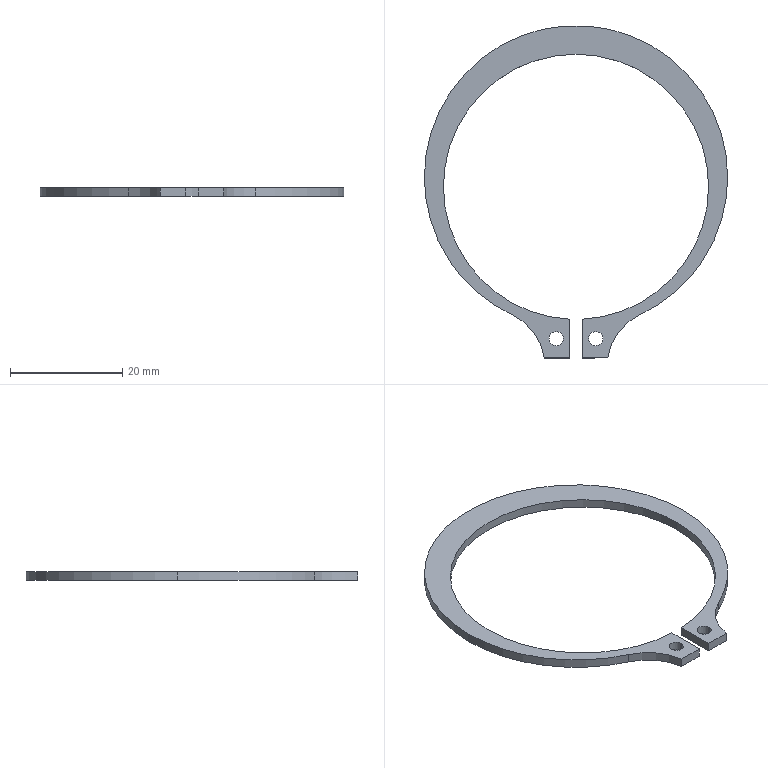Part | SolidWorks | features BaseBody 1 | 1 solid | 18 faces | box 54 x 59.172 x 1.6 mm | volume 946.092 mm3 | cylinder 12 | plane 6 | commonest cylinder face diameters 2.5 x4 47.2 x3 54 x3 19.938 x2
STEP:
#1=CARTESIAN_POINT('',(4.775,-27.022,0.));
#2=VERTEX_POINT('',#1);
#3=CARTESIAN_POINT('',(2.275,-27.022,0.));
#4=VERTEX_POINT('',#3);
#5=CARTESIAN_POINT('',(3.525,-27.022,0.));
#6=DIRECTION('',(0.,0.,-1.));
#7=DIRECTION('',(-1.,0.,0.));
#8=AXIS2_PLACEMENT_3D('',#5,#6,#7);
#9=CIRCLE('',#8,1.25);
#10=EDGE_CURVE('',#2,#4,#9,.T.);
#11=ORIENTED_EDGE('',*,*,#10,.F.);
#12=CARTESIAN_POINT('',(4.775,-27.022,-1.6));
#13=VERTEX_POINT('',#12);
#14=CARTESIAN_POINT('',(4.775,-27.022,0.));
#15=DIRECTION('',(0.,0.,-1.));
#16=VECTOR('',#15,1000.);
#17=LINE('',#14,#16);
#18=EDGE_CURVE('',#2,#13,#17,.T.);
#19=ORIENTED_EDGE('',*,*,#18,.T.);
#20=CARTESIAN_POINT('',(2.275,-27.022,-1.6));
#21=VERTEX_POINT('',#20);
#22=CARTESIAN_POINT('',(3.525,-27.022,-1.6));
#23=DIRECTION('',(0.,0.,-1.));
#24=DIRECTION('',(-1.,0.,0.));
#25=AXIS2_PLACEMENT_3D('',#22,#23,#24);
#26=CIRCLE('',#25,1.25);
#27=EDGE_CURVE('',#13,#21,#26,.T.);
#28=ORIENTED_EDGE('',*,*,#27,.T.);
#29=CARTESIAN_POINT('',(2.275,-27.022,0.));
#30=DIRECTION('',(0.,0.,-1.));
#31=VECTOR('',#30,1000.);
#32=LINE('',#29,#31);
#33=EDGE_CURVE('',#4,#21,#32,.T.);
#34=ORIENTED_EDGE('',*,*,#33,.F.);
#35=EDGE_LOOP('',(#11,#19,#28,#34));
#36=FACE_OUTER_BOUND('',#35,.T.);
#37=CARTESIAN_POINT('',(3.525,-27.022,0.));
#38=DIRECTION('',(0.,0.,-1.));
#39=DIRECTION('',(-1.,0.,0.));
#40=AXIS2_PLACEMENT_3D('',#37,#38,#39);
#41=CYLINDRICAL_SURFACE('',#40,1.25);
#42=ADVANCED_FACE('',(#36),#41,.F.);
#43=CARTESIAN_POINT('',(-2.275,-27.022,0.));
#44=VERTEX_POINT('',#43);
#45=CARTESIAN_POINT('',(-4.775,-27.022,0.));
#46=VERTEX_POINT('',#45);
#47=CARTESIAN_POINT('',(-3.525,-27.022,0.));
#48=DIRECTION('',(0.,0.,-1.));
#49=DIRECTION('',(-1.,0.,0.));
#50=AXIS2_PLACEMENT_3D('',#47,#48,#49);
#51=CIRCLE('',#50,1.25);
#52=EDGE_CURVE('',#44,#46,#51,.T.);
#53=ORIENTED_EDGE('',*,*,#52,.F.);
#54=CARTESIAN_POINT('',(-2.275,-27.022,-1.6));
#55=VERTEX_POINT('',#54);
#56=CARTESIAN_POINT('',(-2.275,-27.022,0.));
#57=DIRECTION('',(0.,0.,-1.));
#58=VECTOR('',#57,1000.);
#59=LINE('',#56,#58);
#60=EDGE_CURVE('',#44,#55,#59,.T.);
#61=ORIENTED_EDGE('',*,*,#60,.T.);
#62=CARTESIAN_POINT('',(-4.775,-27.022,-1.6));
#63=VERTEX_POINT('',#62);
#64=CARTESIAN_POINT('',(-3.525,-27.022,-1.6));
#65=DIRECTION('',(0.,0.,-1.));
#66=DIRECTION('',(-1.,0.,0.));
#67=AXIS2_PLACEMENT_3D('',#64,#65,#66);
#68=CIRCLE('',#67,1.25);
#69=EDGE_CURVE('',#55,#63,#68,.T.);
#70=ORIENTED_EDGE('',*,*,#69,.T.);
#71=CARTESIAN_POINT('',(-4.775,-27.022,0.));
#72=DIRECTION('',(0.,0.,-1.));
#73=VECTOR('',#72,1000.);
#74=LINE('',#71,#73);
#75=EDGE_CURVE('',#46,#63,#74,.T.);
#76=ORIENTED_EDGE('',*,*,#75,.F.);
#77=EDGE_LOOP('',(#53,#61,#70,#76));
#78=FACE_OUTER_BOUND('',#77,.T.);
#79=CARTESIAN_POINT('',(-3.525,-27.022,0.));
#80=DIRECTION('',(0.,0.,-1.));
#81=DIRECTION('',(-1.,0.,0.));
#82=AXIS2_PLACEMENT_3D('',#79,#80,#81);
#83=CYLINDRICAL_SURFACE('',#82,1.25);
#84=ADVANCED_FACE('',(#78),#83,.F.);
#85=CARTESIAN_POINT('',(-27.,1.7,0.));
#86=VERTEX_POINT('',#85);
#87=CARTESIAN_POINT('',(27.,1.7,0.));
#88=VERTEX_POINT('',#87);
#89=CARTESIAN_POINT('',(0.,1.7,0.));
#90=DIRECTION('',(0.,0.,-1.));
#91=DIRECTION('',(-1.,0.,0.));
#92=AXIS2_PLACEMENT_3D('',#89,#90,#91);
#93=CIRCLE('',#92,27.);
#94=EDGE_CURVE('',#86,#88,#93,.T.);
#95=ORIENTED_EDGE('',*,*,#94,.T.);
#96=CARTESIAN_POINT('',(27.,1.7,-1.6));
#97=VERTEX_POINT('',#96);
#98=CARTESIAN_POINT('',(27.,1.7,0.));
#99=DIRECTION('',(0.,0.,-1.));
#100=VECTOR('',#99,1000.);
#101=LINE('',#98,#100);
#102=EDGE_CURVE('',#88,#97,#101,.T.);
#103=ORIENTED_EDGE('',*,*,#102,.T.);
#104=CARTESIAN_POINT('',(-27.,1.7,-1.6));
#105=VERTEX_POINT('',#104);
#106=CARTESIAN_POINT('',(0.,1.7,-1.6));
#107=DIRECTION('',(0.,0.,1.));
#108=DIRECTION('',(-1.,0.,0.));
#109=AXIS2_PLACEMENT_3D('',#106,#107,#108);
#110=CIRCLE('',#109,27.);
#111=EDGE_CURVE('',#97,#105,#110,.T.);
#112=ORIENTED_EDGE('',*,*,#111,.T.);
#113=CARTESIAN_POINT('',(-27.,1.7,0.));
#114=DIRECTION('',(0.,0.,-1.));
#115=VECTOR('',#114,1000.);
#116=LINE('',#113,#115);
#117=EDGE_CURVE('',#86,#105,#116,.T.);
#118=ORIENTED_EDGE('',*,*,#117,.F.);
#119=EDGE_LOOP('',(#95,#103,#112,#118));
#120=FACE_OUTER_BOUND('',#119,.T.);
#121=CARTESIAN_POINT('',(0.,1.7,0.));
#122=DIRECTION('',(0.,0.,-1.));
#123=DIRECTION('',(-1.,0.,0.));
#124=AXIS2_PLACEMENT_3D('',#121,#122,#123);
#125=CYLINDRICAL_SURFACE('',#124,27.);
#126=ADVANCED_FACE('',(#120),#125,.T.);
#127=CARTESIAN_POINT('',(-11.337,-22.805,0.));
#128=VERTEX_POINT('',#127);
#129=CARTESIAN_POINT('',(0.,1.7,0.));
#130=DIRECTION('',(0.,0.,-1.));
#131=DIRECTION('',(-1.,0.,0.));
#132=AXIS2_PLACEMENT_3D('',#129,#130,#131);
#133=CIRCLE('',#132,27.);
#134=EDGE_CURVE('',#128,#86,#133,.T.);
#135=ORIENTED_EDGE('',*,*,#134,.T.);
#136=ORIENTED_EDGE('',*,*,#117,.T.);
#137=CARTESIAN_POINT('',(-11.337,-22.805,-1.6));
#138=VERTEX_POINT('',#137);
#139=CARTESIAN_POINT('',(0.,1.7,-1.6));
#140=DIRECTION('',(0.,0.,1.));
#141=DIRECTION('',(-1.,0.,0.));
#142=AXIS2_PLACEMENT_3D('',#139,#140,#141);
#143=CIRCLE('',#142,27.);
#144=EDGE_CURVE('',#105,#138,#143,.T.);
#145=ORIENTED_EDGE('',*,*,#144,.T.);
#146=CARTESIAN_POINT('',(-11.337,-22.805,0.));
#147=DIRECTION('',(0.,0.,1.));
#148=VECTOR('',#147,1000.);
#149=LINE('',#146,#148);
#150=EDGE_CURVE('',#138,#128,#149,.T.);
#151=ORIENTED_EDGE('',*,*,#150,.T.);
#152=EDGE_LOOP('',(#135,#136,#145,#151));
#153=FACE_OUTER_BOUND('',#152,.T.);
#154=CARTESIAN_POINT('',(0.,1.7,0.));
#155=DIRECTION('',(0.,0.,-1.));
#156=DIRECTION('',(-1.,0.,0.));
#157=AXIS2_PLACEMENT_3D('',#154,#155,#156);
#158=CYLINDRICAL_SURFACE('',#157,27.);
#159=ADVANCED_FACE('',(#153),#158,.T.);
#160=CARTESIAN_POINT('',(23.6,0.,0.));
#161=VERTEX_POINT('',#160);
#162=CARTESIAN_POINT('',(1.15,-23.572,0.));
#163=VERTEX_POINT('',#162);
#164=CARTESIAN_POINT('',(0.,0.,0.));
#165=DIRECTION('',(0.,0.,-1.));
#166=DIRECTION('',(-1.,0.,0.));
#167=AXIS2_PLACEMENT_3D('',#164,#165,#166);
#168=CIRCLE('',#167,23.6);
#169=EDGE_CURVE('',#161,#163,#168,.T.);
#170=ORIENTED_EDGE('',*,*,#169,.F.);
#171=CARTESIAN_POINT('',(23.6,0.,-1.6));
#172=VERTEX_POINT('',#171);
#173=CARTESIAN_POINT('',(23.6,0.,0.));
#174=DIRECTION('',(0.,0.,-1.));
#175=VECTOR('',#174,1000.);
#176=LINE('',#173,#175);
#177=EDGE_CURVE('',#161,#172,#176,.T.);
#178=ORIENTED_EDGE('',*,*,#177,.T.);
#179=CARTESIAN_POINT('',(1.15,-23.572,-1.6));
#180=VERTEX_POINT('',#179);
#181=CARTESIAN_POINT('',(0.,0.,-1.6));
#182=DIRECTION('',(0.,0.,-1.));
#183=DIRECTION('',(-1.,0.,0.));
#184=AXIS2_PLACEMENT_3D('',#181,#182,#183);
#185=CIRCLE('',#184,23.6);
#186=EDGE_CURVE('',#172,#180,#185,.T.);
#187=ORIENTED_EDGE('',*,*,#186,.T.);
#188=CARTESIAN_POINT('',(1.15,-23.572,0.));
#189=DIRECTION('',(0.,0.,-1.));
#190=VECTOR('',#189,1000.);
#191=LINE('',#188,#190);
#192=EDGE_CURVE('',#163,#180,#191,.T.);
#193=ORIENTED_EDGE('',*,*,#192,.F.);
#194=EDGE_LOOP('',(#170,#178,#187,#193));
#195=FACE_OUTER_BOUND('',#194,.T.);
#196=CARTESIAN_POINT('',(0.,0.,0.));
#197=DIRECTION('',(0.,0.,-1.));
#198=DIRECTION('',(-1.,0.,0.));
#199=AXIS2_PLACEMENT_3D('',#196,#197,#198);
#200=CYLINDRICAL_SURFACE('',#199,23.6);
#201=ADVANCED_FACE('',(#195),#200,.F.);
#202=ORIENTED_EDGE('',*,*,#177,.F.);
#203=CARTESIAN_POINT('',(-23.6,0.,0.));
#204=VERTEX_POINT('',#203);
#205=CARTESIAN_POINT('',(0.,0.,0.));
#206=DIRECTION('',(0.,0.,-1.));
#207=DIRECTION('',(-1.,0.,0.));
#208=AXIS2_PLACEMENT_3D('',#205,#206,#207);
#209=CIRCLE('',#208,23.6);
#210=EDGE_CURVE('',#204,#161,#209,.T.);
#211=ORIENTED_EDGE('',*,*,#210,.F.);
#212=CARTESIAN_POINT('',(-23.6,0.,-1.6));
#213=VERTEX_POINT('',#212);
#214=CARTESIAN_POINT('',(-23.6,0.,0.));
#215=DIRECTION('',(0.,0.,-1.));
#216=VECTOR('',#215,1000.);
#217=LINE('',#214,#216);
#218=EDGE_CURVE('',#204,#213,#217,.T.);
#219=ORIENTED_EDGE('',*,*,#218,.T.);
#220=CARTESIAN_POINT('',(0.,0.,-1.6));
#221=DIRECTION('',(0.,0.,-1.));
#222=DIRECTION('',(-1.,0.,0.));
#223=AXIS2_PLACEMENT_3D('',#220,#221,#222);
#224=CIRCLE('',#223,23.6);
#225=EDGE_CURVE('',#213,#172,#224,.T.);
#226=ORIENTED_EDGE('',*,*,#225,.T.);
#227=EDGE_LOOP('',(#202,#211,#219,#226));
#228=FACE_OUTER_BOUND('',#227,.T.);
#229=CARTESIAN_POINT('',(0.,0.,0.));
#230=DIRECTION('',(0.,0.,-1.));
#231=DIRECTION('',(-1.,0.,0.));
#232=AXIS2_PLACEMENT_3D('',#229,#230,#231);
#233=CYLINDRICAL_SURFACE('',#232,23.6);
#234=ADVANCED_FACE('',(#228),#233,.F.);
#235=CARTESIAN_POINT('',(3.525,-27.022,-1.6));
#236=DIRECTION('',(0.,0.,-1.));
#237=DIRECTION('',(-1.,0.,0.));
#238=AXIS2_PLACEMENT_3D('',#235,#236,#237);
#239=CIRCLE('',#238,1.25);
#240=EDGE_CURVE('',#21,#13,#239,.T.);
#241=ORIENTED_EDGE('',*,*,#240,.F.);
#242=ORIENTED_EDGE('',*,*,#27,.F.);
#243=EDGE_LOOP('',(#241,#242));
#244=FACE_BOUND('',#243,.T.);
#245=CARTESIAN_POINT('',(-3.525,-27.022,-1.6));
#246=DIRECTION('',(0.,0.,-1.));
#247=DIRECTION('',(-1.,0.,0.));
#248=AXIS2_PLACEMENT_3D('',#245,#246,#247);
#249=CIRCLE('',#248,1.25);
#250=EDGE_CURVE('',#63,#55,#249,.T.);
#251=ORIENTED_EDGE('',*,*,#250,.F.);
#252=ORIENTED_EDGE('',*,*,#69,.F.);
#253=EDGE_LOOP('',(#251,#252));
#254=FACE_BOUND('',#253,.T.);
#255=CARTESIAN_POINT('',(-5.65,-30.472,-1.6));
#256=VERTEX_POINT('',#255);
#257=CARTESIAN_POINT('',(-1.15,-30.472,-1.6));
#258=VERTEX_POINT('',#257);
#259=CARTESIAN_POINT('',(0.,-30.472,-1.6));
#260=DIRECTION('',(1.,0.,0.));
#261=VECTOR('',#260,1000.);
#262=LINE('',#259,#261);
#263=EDGE_CURVE('',#256,#258,#262,.T.);
#264=ORIENTED_EDGE('',*,*,#263,.F.);
#265=CARTESIAN_POINT('',(-15.523,-31.852,-1.6));
#266=DIRECTION('',(0.,0.,-1.));
#267=DIRECTION('',(-1.,0.,0.));
#268=AXIS2_PLACEMENT_3D('',#265,#266,#267);
#269=CIRCLE('',#268,9.969);
#270=EDGE_CURVE('',#138,#256,#269,.T.);
#271=ORIENTED_EDGE('',*,*,#270,.F.);
#272=ORIENTED_EDGE('',*,*,#144,.F.);
#273=ORIENTED_EDGE('',*,*,#111,.F.);
#274=CARTESIAN_POINT('',(11.337,-22.805,-1.6));
#275=VERTEX_POINT('',#274);
#276=CARTESIAN_POINT('',(0.,1.7,-1.6));
#277=DIRECTION('',(0.,0.,1.));
#278=DIRECTION('',(-1.,0.,0.));
#279=AXIS2_PLACEMENT_3D('',#276,#277,#278);
#280=CIRCLE('',#279,27.);
#281=EDGE_CURVE('',#275,#97,#280,.T.);
#282=ORIENTED_EDGE('',*,*,#281,.F.);
#283=CARTESIAN_POINT('',(5.65,-30.472,-1.6));
#284=VERTEX_POINT('',#283);
#285=CARTESIAN_POINT('',(15.523,-31.852,-1.6));
#286=DIRECTION('',(0.,0.,-1.));
#287=DIRECTION('',(-1.,0.,0.));
#288=AXIS2_PLACEMENT_3D('',#285,#286,#287);
#289=CIRCLE('',#288,9.969);
#290=EDGE_CURVE('',#284,#275,#289,.T.);
#291=ORIENTED_EDGE('',*,*,#290,.F.);
#292=CARTESIAN_POINT('',(1.15,-30.472,-1.6));
#293=VERTEX_POINT('',#292);
#294=CARTESIAN_POINT('',(0.,-30.472,-1.6));
#295=DIRECTION('',(1.,0.,0.));
#296=VECTOR('',#295,1000.);
#297=LINE('',#294,#296);
#298=EDGE_CURVE('',#293,#284,#297,.T.);
#299=ORIENTED_EDGE('',*,*,#298,.F.);
#300=CARTESIAN_POINT('',(1.15,-2.891,-1.6));
#301=DIRECTION('',(0.,-1.,0.));
#302=VECTOR('',#301,1000.);
#303=LINE('',#300,#302);
#304=EDGE_CURVE('',#180,#293,#303,.T.);
#305=ORIENTED_EDGE('',*,*,#304,.F.);
#306=ORIENTED_EDGE('',*,*,#186,.F.);
#307=ORIENTED_EDGE('',*,*,#225,.F.);
#308=CARTESIAN_POINT('',(-1.15,-23.572,-1.6));
#309=VERTEX_POINT('',#308);
#310=CARTESIAN_POINT('',(0.,0.,-1.6));
#311=DIRECTION('',(0.,0.,-1.));
#312=DIRECTION('',(-1.,0.,0.));
#313=AXIS2_PLACEMENT_3D('',#310,#311,#312);
#314=CIRCLE('',#313,23.6);
#315=EDGE_CURVE('',#309,#213,#314,.T.);
#316=ORIENTED_EDGE('',*,*,#315,.F.);
#317=CARTESIAN_POINT('',(-1.15,-2.891,-1.6));
#318=DIRECTION('',(0.,1.,0.));
#319=VECTOR('',#318,1000.);
#320=LINE('',#317,#319);
#321=EDGE_CURVE('',#258,#309,#320,.T.);
#322=ORIENTED_EDGE('',*,*,#321,.F.);
#323=EDGE_LOOP('',(#264,#271,#272,#273,#282,#291,#299,#305,#306,#307,#316,#322));
#324=FACE_OUTER_BOUND('',#323,.T.);
#325=CARTESIAN_POINT('',(0.,-2.891,-1.6));
#326=DIRECTION('',(0.,0.,1.));
#327=DIRECTION('',(1.,0.,0.));
#328=AXIS2_PLACEMENT_3D('',#325,#326,#327);
#329=PLANE('',#328);
#330=ADVANCED_FACE('',(#244,#254,#324),#329,.F.);
#331=ORIENTED_EDGE('',*,*,#18,.F.);
#332=CARTESIAN_POINT('',(3.525,-27.022,0.));
#333=DIRECTION('',(0.,0.,-1.));
#334=DIRECTION('',(-1.,0.,0.));
#335=AXIS2_PLACEMENT_3D('',#332,#333,#334);
#336=CIRCLE('',#335,1.25);
#337=EDGE_CURVE('',#4,#2,#336,.T.);
#338=ORIENTED_EDGE('',*,*,#337,.F.);
#339=ORIENTED_EDGE('',*,*,#33,.T.);
#340=ORIENTED_EDGE('',*,*,#240,.T.);
#341=EDGE_LOOP('',(#331,#338,#339,#340));
#342=FACE_OUTER_BOUND('',#341,.T.);
#343=CARTESIAN_POINT('',(3.525,-27.022,0.));
#344=DIRECTION('',(0.,0.,-1.));
#345=DIRECTION('',(-1.,0.,0.));
#346=AXIS2_PLACEMENT_3D('',#343,#344,#345);
#347=CYLINDRICAL_SURFACE('',#346,1.25);
#348=ADVANCED_FACE('',(#342),#347,.F.);
#349=ORIENTED_EDGE('',*,*,#60,.F.);
#350=CARTESIAN_POINT('',(-3.525,-27.022,0.));
#351=DIRECTION('',(0.,0.,-1.));
#352=DIRECTION('',(-1.,0.,0.));
#353=AXIS2_PLACEMENT_3D('',#350,#351,#352);
#354=CIRCLE('',#353,1.25);
#355=EDGE_CURVE('',#46,#44,#354,.T.);
#356=ORIENTED_EDGE('',*,*,#355,.F.);
#357=ORIENTED_EDGE('',*,*,#75,.T.);
#358=ORIENTED_EDGE('',*,*,#250,.T.);
#359=EDGE_LOOP('',(#349,#356,#357,#358));
#360=FACE_OUTER_BOUND('',#359,.T.);
#361=CARTESIAN_POINT('',(-3.525,-27.022,0.));
#362=DIRECTION('',(0.,0.,-1.));
#363=DIRECTION('',(-1.,0.,0.));
#364=AXIS2_PLACEMENT_3D('',#361,#362,#363);
#365=CYLINDRICAL_SURFACE('',#364,1.25);
#366=ADVANCED_FACE('',(#360),#365,.F.);
#367=CARTESIAN_POINT('',(-1.15,-23.572,0.));
#368=VERTEX_POINT('',#367);
#369=CARTESIAN_POINT('',(-1.15,-30.472,0.));
#370=VERTEX_POINT('',#369);
#371=CARTESIAN_POINT('',(-1.15,-30.472,0.));
#372=DIRECTION('',(0.,-1.,0.));
#373=VECTOR('',#372,1000.);
#374=LINE('',#371,#373);
#375=EDGE_CURVE('',#368,#370,#374,.T.);
#376=ORIENTED_EDGE('',*,*,#375,.T.);
#377=CARTESIAN_POINT('',(-1.15,-30.472,0.));
#378=DIRECTION('',(0.,0.,-1.));
#379=VECTOR('',#378,1000.);
#380=LINE('',#377,#379);
#381=EDGE_CURVE('',#370,#258,#380,.T.);
#382=ORIENTED_EDGE('',*,*,#381,.T.);
#383=ORIENTED_EDGE('',*,*,#321,.T.);
#384=CARTESIAN_POINT('',(-1.15,-23.572,0.));
#385=DIRECTION('',(0.,0.,1.));
#386=VECTOR('',#385,1000.);
#387=LINE('',#384,#386);
#388=EDGE_CURVE('',#309,#368,#387,.T.);
#389=ORIENTED_EDGE('',*,*,#388,.T.);
#390=EDGE_LOOP('',(#376,#382,#383,#389));
#391=FACE_OUTER_BOUND('',#390,.T.);
#392=CARTESIAN_POINT('',(-1.15,-30.472,0.));
#393=DIRECTION('',(1.,0.,0.));
#394=DIRECTION('',(0.,1.,0.));
#395=AXIS2_PLACEMENT_3D('',#392,#393,#394);
#396=PLANE('',#395);
#397=ADVANCED_FACE('',(#391),#396,.T.);
#398=CARTESIAN_POINT('',(-5.65,-30.472,0.));
#399=VERTEX_POINT('',#398);
#400=CARTESIAN_POINT('',(-5.65,-30.472,0.));
#401=DIRECTION('',(-1.,0.,0.));
#402=VECTOR('',#401,1000.);
#403=LINE('',#400,#402);
#404=EDGE_CURVE('',#370,#399,#403,.T.);
#405=ORIENTED_EDGE('',*,*,#404,.T.);
#406=CARTESIAN_POINT('',(-5.65,-30.472,0.));
#407=DIRECTION('',(0.,0.,-1.));
#408=VECTOR('',#407,1000.);
#409=LINE('',#406,#408);
#410=EDGE_CURVE('',#399,#256,#409,.T.);
#411=ORIENTED_EDGE('',*,*,#410,.T.);
#412=ORIENTED_EDGE('',*,*,#263,.T.);
#413=ORIENTED_EDGE('',*,*,#381,.F.);
#414=EDGE_LOOP('',(#405,#411,#412,#413));
#415=FACE_OUTER_BOUND('',#414,.T.);
#416=CARTESIAN_POINT('',(-5.65,-30.472,0.));
#417=DIRECTION('',(0.,-1.,0.));
#418=DIRECTION('',(0.,0.,-1.));
#419=AXIS2_PLACEMENT_3D('',#416,#417,#418);
#420=PLANE('',#419);
#421=ADVANCED_FACE('',(#415),#420,.T.);
#422=ORIENTED_EDGE('',*,*,#410,.F.);
#423=CARTESIAN_POINT('',(-15.523,-31.852,0.));
#424=DIRECTION('',(0.,0.,-1.));
#425=DIRECTION('',(-1.,0.,0.));
#426=AXIS2_PLACEMENT_3D('',#423,#424,#425);
#427=CIRCLE('',#426,9.969);
#428=EDGE_CURVE('',#128,#399,#427,.T.);
#429=ORIENTED_EDGE('',*,*,#428,.F.);
#430=ORIENTED_EDGE('',*,*,#150,.F.);
#431=ORIENTED_EDGE('',*,*,#270,.T.);
#432=EDGE_LOOP('',(#422,#429,#430,#431));
#433=FACE_OUTER_BOUND('',#432,.T.);
#434=CARTESIAN_POINT('',(-15.523,-31.852,0.));
#435=DIRECTION('',(0.,0.,-1.));
#436=DIRECTION('',(-1.,0.,0.));
#437=AXIS2_PLACEMENT_3D('',#434,#435,#436);
#438=CYLINDRICAL_SURFACE('',#437,9.969);
#439=ADVANCED_FACE('',(#433),#438,.F.);
#440=ORIENTED_EDGE('',*,*,#102,.F.);
#441=CARTESIAN_POINT('',(11.337,-22.805,0.));
#442=VERTEX_POINT('',#441);
#443=CARTESIAN_POINT('',(0.,1.7,0.));
#444=DIRECTION('',(0.,0.,-1.));
#445=DIRECTION('',(-1.,0.,0.));
#446=AXIS2_PLACEMENT_3D('',#443,#444,#445);
#447=CIRCLE('',#446,27.);
#448=EDGE_CURVE('',#88,#442,#447,.T.);
#449=ORIENTED_EDGE('',*,*,#448,.T.);
#450=CARTESIAN_POINT('',(11.337,-22.805,0.));
#451=DIRECTION('',(0.,0.,-1.));
#452=VECTOR('',#451,1000.);
#453=LINE('',#450,#452);
#454=EDGE_CURVE('',#442,#275,#453,.T.);
#455=ORIENTED_EDGE('',*,*,#454,.T.);
#456=ORIENTED_EDGE('',*,*,#281,.T.);
#457=EDGE_LOOP('',(#440,#449,#455,#456));
#458=FACE_OUTER_BOUND('',#457,.T.);
#459=CARTESIAN_POINT('',(0.,1.7,0.));
#460=DIRECTION('',(0.,0.,-1.));
#461=DIRECTION('',(-1.,0.,0.));
#462=AXIS2_PLACEMENT_3D('',#459,#460,#461);
#463=CYLINDRICAL_SURFACE('',#462,27.);
#464=ADVANCED_FACE('',(#458),#463,.T.);
#465=ORIENTED_EDGE('',*,*,#454,.F.);
#466=CARTESIAN_POINT('',(5.65,-30.472,0.));
#467=VERTEX_POINT('',#466);
#468=CARTESIAN_POINT('',(15.523,-31.852,0.));
#469=DIRECTION('',(0.,0.,-1.));
#470=DIRECTION('',(-1.,0.,0.));
#471=AXIS2_PLACEMENT_3D('',#468,#469,#470);
#472=CIRCLE('',#471,9.969);
#473=EDGE_CURVE('',#467,#442,#472,.T.);
#474=ORIENTED_EDGE('',*,*,#473,.F.);
#475=CARTESIAN_POINT('',(5.65,-30.472,0.));
#476=DIRECTION('',(0.,0.,1.));
#477=VECTOR('',#476,1000.);
#478=LINE('',#475,#477);
#479=EDGE_CURVE('',#284,#467,#478,.T.);
#480=ORIENTED_EDGE('',*,*,#479,.F.);
#481=ORIENTED_EDGE('',*,*,#290,.T.);
#482=EDGE_LOOP('',(#465,#474,#480,#481));
#483=FACE_OUTER_BOUND('',#482,.T.);
#484=CARTESIAN_POINT('',(15.523,-31.852,0.));
#485=DIRECTION('',(0.,0.,-1.));
#486=DIRECTION('',(-1.,0.,0.));
#487=AXIS2_PLACEMENT_3D('',#484,#485,#486);
#488=CYLINDRICAL_SURFACE('',#487,9.969);
#489=ADVANCED_FACE('',(#483),#488,.F.);
#490=CARTESIAN_POINT('',(1.15,-30.472,0.));
#491=VERTEX_POINT('',#490);
#492=CARTESIAN_POINT('',(1.15,-30.472,0.));
#493=DIRECTION('',(-1.,0.,0.));
#494=VECTOR('',#493,1000.);
#495=LINE('',#492,#494);
#496=EDGE_CURVE('',#467,#491,#495,.T.);
#497=ORIENTED_EDGE('',*,*,#496,.T.);
#498=CARTESIAN_POINT('',(1.15,-30.472,0.));
#499=DIRECTION('',(0.,0.,-1.));
#500=VECTOR('',#499,1000.);
#501=LINE('',#498,#500);
#502=EDGE_CURVE('',#491,#293,#501,.T.);
#503=ORIENTED_EDGE('',*,*,#502,.T.);
#504=ORIENTED_EDGE('',*,*,#298,.T.);
#505=ORIENTED_EDGE('',*,*,#479,.T.);
#506=EDGE_LOOP('',(#497,#503,#504,#505));
#507=FACE_OUTER_BOUND('',#506,.T.);
#508=CARTESIAN_POINT('',(1.15,-30.472,0.));
#509=DIRECTION('',(0.,-1.,0.));
#510=DIRECTION('',(0.,0.,-1.));
#511=AXIS2_PLACEMENT_3D('',#508,#509,#510);
#512=PLANE('',#511);
#513=ADVANCED_FACE('',(#507),#512,.T.);
#514=CARTESIAN_POINT('',(1.15,-23.572,0.));
#515=DIRECTION('',(0.,1.,0.));
#516=VECTOR('',#515,1000.);
#517=LINE('',#514,#516);
#518=EDGE_CURVE('',#491,#163,#517,.T.);
#519=ORIENTED_EDGE('',*,*,#518,.T.);
#520=ORIENTED_EDGE('',*,*,#192,.T.);
#521=ORIENTED_EDGE('',*,*,#304,.T.);
#522=ORIENTED_EDGE('',*,*,#502,.F.);
#523=EDGE_LOOP('',(#519,#520,#521,#522));
#524=FACE_OUTER_BOUND('',#523,.T.);
#525=CARTESIAN_POINT('',(1.15,-23.572,0.));
#526=DIRECTION('',(-1.,0.,0.));
#527=DIRECTION('',(0.,-1.,0.));
#528=AXIS2_PLACEMENT_3D('',#525,#526,#527);
#529=PLANE('',#528);
#530=ADVANCED_FACE('',(#524),#529,.T.);
#531=ORIENTED_EDGE('',*,*,#218,.F.);
#532=CARTESIAN_POINT('',(0.,0.,0.));
#533=DIRECTION('',(0.,0.,-1.));
#534=DIRECTION('',(-1.,0.,0.));
#535=AXIS2_PLACEMENT_3D('',#532,#533,#534);
#536=CIRCLE('',#535,23.6);
#537=EDGE_CURVE('',#368,#204,#536,.T.);
#538=ORIENTED_EDGE('',*,*,#537,.F.);
#539=ORIENTED_EDGE('',*,*,#388,.F.);
#540=ORIENTED_EDGE('',*,*,#315,.T.);
#541=EDGE_LOOP('',(#531,#538,#539,#540));
#542=FACE_OUTER_BOUND('',#541,.T.);
#543=CARTESIAN_POINT('',(0.,0.,0.));
#544=DIRECTION('',(0.,0.,-1.));
#545=DIRECTION('',(-1.,0.,0.));
#546=AXIS2_PLACEMENT_3D('',#543,#544,#545);
#547=CYLINDRICAL_SURFACE('',#546,23.6);
#548=ADVANCED_FACE('',(#542),#547,.F.);
#549=ORIENTED_EDGE('',*,*,#337,.T.);
#550=ORIENTED_EDGE('',*,*,#10,.T.);
#551=EDGE_LOOP('',(#549,#550));
#552=FACE_BOUND('',#551,.T.);
#553=ORIENTED_EDGE('',*,*,#355,.T.);
#554=ORIENTED_EDGE('',*,*,#52,.T.);
#555=EDGE_LOOP('',(#553,#554));
#556=FACE_BOUND('',#555,.T.);
#557=ORIENTED_EDGE('',*,*,#134,.F.);
#558=ORIENTED_EDGE('',*,*,#428,.T.);
#559=ORIENTED_EDGE('',*,*,#404,.F.);
#560=ORIENTED_EDGE('',*,*,#375,.F.);
#561=ORIENTED_EDGE('',*,*,#537,.T.);
#562=ORIENTED_EDGE('',*,*,#210,.T.);
#563=ORIENTED_EDGE('',*,*,#169,.T.);
#564=ORIENTED_EDGE('',*,*,#518,.F.);
#565=ORIENTED_EDGE('',*,*,#496,.F.);
#566=ORIENTED_EDGE('',*,*,#473,.T.);
#567=ORIENTED_EDGE('',*,*,#448,.F.);
#568=ORIENTED_EDGE('',*,*,#94,.F.);
#569=EDGE_LOOP('',(#557,#558,#559,#560,#561,#562,#563,#564,#565,#566,#567,#568));
#570=FACE_OUTER_BOUND('',#569,.T.);
#571=CARTESIAN_POINT('',(0.,-2.891,0.));
#572=DIRECTION('',(0.,0.,1.));
#573=DIRECTION('',(1.,0.,0.));
#574=AXIS2_PLACEMENT_3D('',#571,#572,#573);
#575=PLANE('',#574);
#576=ADVANCED_FACE('',(#552,#556,#570),#575,.T.);
#577=CLOSED_SHELL('',(#42,#84,#126,#159,#201,#234,#330,#348,#366,#397,#421,#439,#464,#489,#513,#530,#548,#576));
#578=MANIFOLD_SOLID_BREP('',#577);
#579=CARTESIAN_POINT('',(0.,0.,0.));
#580=DIRECTION('',(0.,0.,1.));
#581=DIRECTION('',(1.,0.,0.));
#582=AXIS2_PLACEMENT_3D('',#579,#580,#581);
#583=(LENGTH_UNIT()NAMED_UNIT(*)SI_UNIT(.MILLI.,.METRE.));
#584=UNCERTAINTY_MEASURE_WITH_UNIT(LENGTH_MEASURE(0.00001),#583,'','');
#585=(NAMED_UNIT(*)PLANE_ANGLE_UNIT()SI_UNIT($,.RADIAN.));
#586=(NAMED_UNIT(*)SI_UNIT($,.STERADIAN.)SOLID_ANGLE_UNIT());
#587=(GEOMETRIC_REPRESENTATION_CONTEXT(3)GLOBAL_UNCERTAINTY_ASSIGNED_CONTEXT((#584))GLOBAL_UNIT_ASSIGNED_CONTEXT((#583,#585,#586))REPRESENTATION_CONTEXT('',''));
#588=ADVANCED_BREP_SHAPE_REPRESENTATION('',(#578,#582),#587);